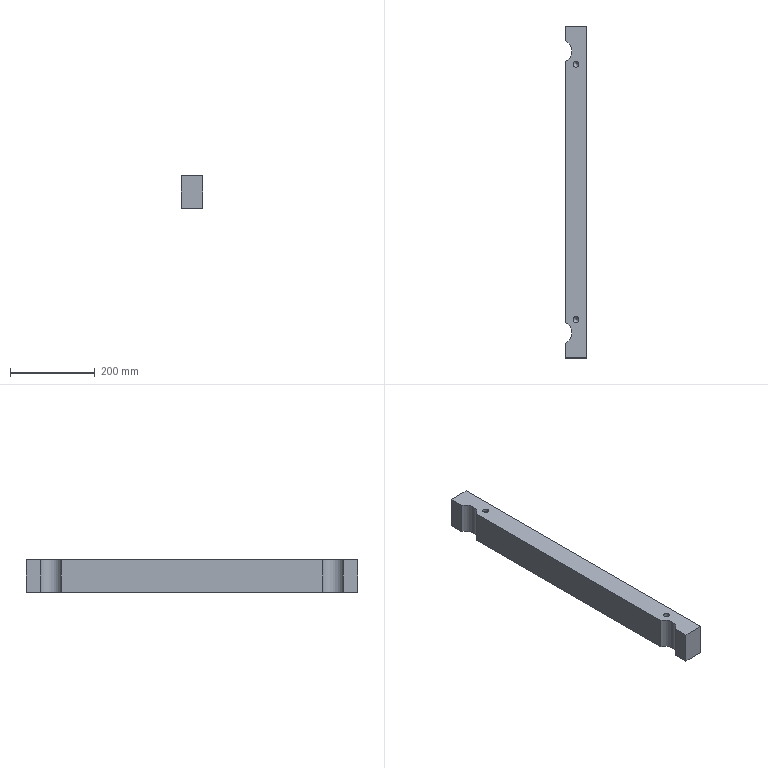Part | NX | features 3 2 | 1 solid | 14 faces | box 50 x 782.437 x 75.5 mm | volume 2869350 mm3 | plane 8 | cylinder 4 | cone 2 | commonest cylinder face diameters 14.1 x2 53 x2
STEP:
#1=CARTESIAN_POINT('',(2467.05,301.218,256.5));
#2=VERTEX_POINT('',#1);
#3=CARTESIAN_POINT('',(2460.,301.218,256.5));
#4=DIRECTION('',(0.,0.,-1.));
#5=DIRECTION('',(1.,0.,0.));
#6=AXIS2_PLACEMENT_3D('',#3,#4,#5);
#7=CIRCLE('',#6,7.05);
#8=EDGE_CURVE('',#2,#2,#7,.T.);
#9=ORIENTED_EDGE('',*,*,#8,.T.);
#10=EDGE_LOOP('',(#9));
#11=FACE_BOUND('',#10,.T.);
#12=CARTESIAN_POINT('',(2435.,-307.891,256.5));
#13=VERTEX_POINT('',#12);
#14=CARTESIAN_POINT('',(2435.,-356.109,256.5));
#15=VERTEX_POINT('',#14);
#16=CARTESIAN_POINT('',(2424.,-332.,256.5));
#17=DIRECTION('',(0.,0.,-1.));
#18=DIRECTION('',(1.,0.,0.));
#19=AXIS2_PLACEMENT_3D('',#16,#17,#18);
#20=CIRCLE('',#19,26.5);
#21=EDGE_CURVE('',#13,#15,#20,.T.);
#22=ORIENTED_EDGE('',*,*,#21,.T.);
#23=CARTESIAN_POINT('',(2435.,-391.218,256.5));
#24=VERTEX_POINT('',#23);
#25=CARTESIAN_POINT('',(2435.,193.,256.5));
#26=DIRECTION('',(0.,1.,0.));
#27=VECTOR('',#26,1000.);
#28=LINE('',#25,#27);
#29=EDGE_CURVE('',#24,#15,#28,.T.);
#30=ORIENTED_EDGE('',*,*,#29,.F.);
#31=CARTESIAN_POINT('',(2485.,-391.218,256.5));
#32=VERTEX_POINT('',#31);
#33=CARTESIAN_POINT('',(4475.,-391.218,256.5));
#34=DIRECTION('',(1.,0.,0.));
#35=VECTOR('',#34,1000.);
#36=LINE('',#33,#35);
#37=EDGE_CURVE('',#24,#32,#36,.T.);
#38=ORIENTED_EDGE('',*,*,#37,.T.);
#39=CARTESIAN_POINT('',(2485.,391.218,256.5));
#40=VERTEX_POINT('',#39);
#41=CARTESIAN_POINT('',(2485.,193.,256.5));
#42=DIRECTION('',(0.,-1.,0.));
#43=VECTOR('',#42,1000.);
#44=LINE('',#41,#43);
#45=EDGE_CURVE('',#40,#32,#44,.T.);
#46=ORIENTED_EDGE('',*,*,#45,.F.);
#47=CARTESIAN_POINT('',(2435.,391.218,256.5));
#48=VERTEX_POINT('',#47);
#49=CARTESIAN_POINT('',(4475.,391.218,256.5));
#50=DIRECTION('',(1.,0.,0.));
#51=VECTOR('',#50,1000.);
#52=LINE('',#49,#51);
#53=EDGE_CURVE('',#48,#40,#52,.T.);
#54=ORIENTED_EDGE('',*,*,#53,.F.);
#55=CARTESIAN_POINT('',(2435.,356.109,256.5));
#56=VERTEX_POINT('',#55);
#57=CARTESIAN_POINT('',(2435.,193.,256.5));
#58=DIRECTION('',(0.,1.,0.));
#59=VECTOR('',#58,1000.);
#60=LINE('',#57,#59);
#61=EDGE_CURVE('',#56,#48,#60,.T.);
#62=ORIENTED_EDGE('',*,*,#61,.F.);
#63=CARTESIAN_POINT('',(2435.,307.891,256.5));
#64=VERTEX_POINT('',#63);
#65=CARTESIAN_POINT('',(2424.,332.,256.5));
#66=DIRECTION('',(0.,0.,1.));
#67=DIRECTION('',(1.,0.,0.));
#68=AXIS2_PLACEMENT_3D('',#65,#66,#67);
#69=CIRCLE('',#68,26.5);
#70=EDGE_CURVE('',#64,#56,#69,.T.);
#71=ORIENTED_EDGE('',*,*,#70,.F.);
#72=CARTESIAN_POINT('',(2435.,193.,256.5));
#73=DIRECTION('',(0.,1.,0.));
#74=VECTOR('',#73,1000.);
#75=LINE('',#72,#74);
#76=EDGE_CURVE('',#13,#64,#75,.T.);
#77=ORIENTED_EDGE('',*,*,#76,.F.);
#78=EDGE_LOOP('',(#22,#30,#38,#46,#54,#62,#71,#77));
#79=FACE_BOUND('',#78,.T.);
#80=CARTESIAN_POINT('',(2467.05,-301.218,256.5));
#81=VERTEX_POINT('',#80);
#82=CARTESIAN_POINT('',(2460.,-301.218,256.5));
#83=DIRECTION('',(0.,0.,-1.));
#84=DIRECTION('',(1.,0.,0.));
#85=AXIS2_PLACEMENT_3D('',#82,#83,#84);
#86=CIRCLE('',#85,7.05);
#87=EDGE_CURVE('',#81,#81,#86,.T.);
#88=ORIENTED_EDGE('',*,*,#87,.T.);
#89=EDGE_LOOP('',(#88));
#90=FACE_BOUND('',#89,.T.);
#91=CARTESIAN_POINT('',(4475.,0.,256.5));
#92=DIRECTION('',(0.,0.,1.));
#93=DIRECTION('',(-1.,0.,0.));
#94=AXIS2_PLACEMENT_3D('',#91,#92,#93);
#95=PLANE('',#94);
#96=ADVANCED_FACE('',(#11,#79,#90),#95,.T.);
#97=CARTESIAN_POINT('',(2435.,-356.109,181.));
#98=VERTEX_POINT('',#97);
#99=CARTESIAN_POINT('',(2435.,-356.109,-181.));
#100=DIRECTION('',(0.,0.,-1.));
#101=VECTOR('',#100,1000.);
#102=LINE('',#99,#101);
#103=EDGE_CURVE('',#15,#98,#102,.T.);
#104=ORIENTED_EDGE('',*,*,#103,.T.);
#105=CARTESIAN_POINT('',(2435.,-391.218,181.));
#106=VERTEX_POINT('',#105);
#107=CARTESIAN_POINT('',(2435.,193.,181.));
#108=DIRECTION('',(0.,-1.,0.));
#109=VECTOR('',#108,1000.);
#110=LINE('',#107,#109);
#111=EDGE_CURVE('',#98,#106,#110,.T.);
#112=ORIENTED_EDGE('',*,*,#111,.T.);
#113=CARTESIAN_POINT('',(2435.,-391.218,-1.5));
#114=DIRECTION('',(0.,0.,1.));
#115=VECTOR('',#114,1000.);
#116=LINE('',#113,#115);
#117=EDGE_CURVE('',#106,#24,#116,.T.);
#118=ORIENTED_EDGE('',*,*,#117,.T.);
#119=ORIENTED_EDGE('',*,*,#29,.T.);
#120=EDGE_LOOP('',(#104,#112,#118,#119));
#121=FACE_BOUND('',#120,.T.);
#122=CARTESIAN_POINT('',(2435.,193.,-1.5));
#123=DIRECTION('',(-1.,0.,0.));
#124=DIRECTION('',(0.,0.,-1.));
#125=AXIS2_PLACEMENT_3D('',#122,#123,#124);
#126=PLANE('',#125);
#127=ADVANCED_FACE('',(#121),#126,.T.);
#128=CARTESIAN_POINT('',(2435.,-307.891,181.));
#129=VERTEX_POINT('',#128);
#130=CARTESIAN_POINT('',(2435.,-307.891,181.));
#131=DIRECTION('',(0.,0.,1.));
#132=VECTOR('',#131,1000.);
#133=LINE('',#130,#132);
#134=EDGE_CURVE('',#129,#13,#133,.T.);
#135=ORIENTED_EDGE('',*,*,#134,.T.);
#136=ORIENTED_EDGE('',*,*,#76,.T.);
#137=CARTESIAN_POINT('',(2435.,307.891,181.));
#138=VERTEX_POINT('',#137);
#139=CARTESIAN_POINT('',(2435.,307.891,-181.));
#140=DIRECTION('',(0.,0.,-1.));
#141=VECTOR('',#140,1000.);
#142=LINE('',#139,#141);
#143=EDGE_CURVE('',#64,#138,#142,.T.);
#144=ORIENTED_EDGE('',*,*,#143,.T.);
#145=CARTESIAN_POINT('',(2435.,193.,181.));
#146=DIRECTION('',(0.,-1.,0.));
#147=VECTOR('',#146,1000.);
#148=LINE('',#145,#147);
#149=EDGE_CURVE('',#138,#129,#148,.T.);
#150=ORIENTED_EDGE('',*,*,#149,.T.);
#151=EDGE_LOOP('',(#135,#136,#144,#150));
#152=FACE_BOUND('',#151,.T.);
#153=CARTESIAN_POINT('',(2435.,193.,-1.5));
#154=DIRECTION('',(-1.,0.,0.));
#155=DIRECTION('',(0.,0.,-1.));
#156=AXIS2_PLACEMENT_3D('',#153,#154,#155);
#157=PLANE('',#156);
#158=ADVANCED_FACE('',(#152),#157,.T.);
#159=CARTESIAN_POINT('',(2435.,356.109,181.));
#160=VERTEX_POINT('',#159);
#161=CARTESIAN_POINT('',(2435.,356.109,181.));
#162=DIRECTION('',(0.,0.,1.));
#163=VECTOR('',#162,1000.);
#164=LINE('',#161,#163);
#165=EDGE_CURVE('',#160,#56,#164,.T.);
#166=ORIENTED_EDGE('',*,*,#165,.T.);
#167=ORIENTED_EDGE('',*,*,#61,.T.);
#168=CARTESIAN_POINT('',(2435.,391.218,181.));
#169=VERTEX_POINT('',#168);
#170=CARTESIAN_POINT('',(2435.,391.218,-1.5));
#171=DIRECTION('',(0.,0.,1.));
#172=VECTOR('',#171,1000.);
#173=LINE('',#170,#172);
#174=EDGE_CURVE('',#169,#48,#173,.T.);
#175=ORIENTED_EDGE('',*,*,#174,.F.);
#176=CARTESIAN_POINT('',(2435.,193.,181.));
#177=DIRECTION('',(0.,-1.,0.));
#178=VECTOR('',#177,1000.);
#179=LINE('',#176,#178);
#180=EDGE_CURVE('',#169,#160,#179,.T.);
#181=ORIENTED_EDGE('',*,*,#180,.T.);
#182=EDGE_LOOP('',(#166,#167,#175,#181));
#183=FACE_BOUND('',#182,.T.);
#184=CARTESIAN_POINT('',(2435.,193.,-1.5));
#185=DIRECTION('',(-1.,0.,0.));
#186=DIRECTION('',(0.,0.,-1.));
#187=AXIS2_PLACEMENT_3D('',#184,#185,#186);
#188=PLANE('',#187);
#189=ADVANCED_FACE('',(#183),#188,.T.);
#190=CARTESIAN_POINT('',(2485.,-391.218,181.));
#191=VERTEX_POINT('',#190);
#192=CARTESIAN_POINT('',(2485.,391.218,181.));
#193=VERTEX_POINT('',#192);
#194=CARTESIAN_POINT('',(2485.,193.,181.));
#195=DIRECTION('',(0.,1.,0.));
#196=VECTOR('',#195,1000.);
#197=LINE('',#194,#196);
#198=EDGE_CURVE('',#191,#193,#197,.T.);
#199=ORIENTED_EDGE('',*,*,#198,.T.);
#200=CARTESIAN_POINT('',(2485.,391.218,-1.5));
#201=DIRECTION('',(0.,0.,-1.));
#202=VECTOR('',#201,1000.);
#203=LINE('',#200,#202);
#204=EDGE_CURVE('',#40,#193,#203,.T.);
#205=ORIENTED_EDGE('',*,*,#204,.F.);
#206=ORIENTED_EDGE('',*,*,#45,.T.);
#207=CARTESIAN_POINT('',(2485.,-391.218,-1.5));
#208=DIRECTION('',(0.,0.,-1.));
#209=VECTOR('',#208,1000.);
#210=LINE('',#207,#209);
#211=EDGE_CURVE('',#32,#191,#210,.T.);
#212=ORIENTED_EDGE('',*,*,#211,.T.);
#213=EDGE_LOOP('',(#199,#205,#206,#212));
#214=FACE_BOUND('',#213,.T.);
#215=CARTESIAN_POINT('',(2485.,193.,-1.5));
#216=DIRECTION('',(1.,0.,0.));
#217=DIRECTION('',(0.,0.,1.));
#218=AXIS2_PLACEMENT_3D('',#215,#216,#217);
#219=PLANE('',#218);
#220=ADVANCED_FACE('',(#214),#219,.T.);
#221=CARTESIAN_POINT('',(2424.,-332.,181.));
#222=DIRECTION('',(0.,0.,-1.));
#223=DIRECTION('',(-1.,0.,0.));
#224=AXIS2_PLACEMENT_3D('',#221,#222,#223);
#225=CIRCLE('',#224,26.5);
#226=EDGE_CURVE('',#129,#98,#225,.T.);
#227=ORIENTED_EDGE('',*,*,#226,.F.);
#228=ORIENTED_EDGE('',*,*,#149,.F.);
#229=CARTESIAN_POINT('',(2424.,332.,181.));
#230=DIRECTION('',(0.,0.,1.));
#231=DIRECTION('',(-1.,0.,0.));
#232=AXIS2_PLACEMENT_3D('',#229,#230,#231);
#233=CIRCLE('',#232,26.5);
#234=EDGE_CURVE('',#138,#160,#233,.T.);
#235=ORIENTED_EDGE('',*,*,#234,.T.);
#236=ORIENTED_EDGE('',*,*,#180,.F.);
#237=CARTESIAN_POINT('',(3705.,391.218,181.));
#238=DIRECTION('',(-1.,0.,0.));
#239=VECTOR('',#238,1000.);
#240=LINE('',#237,#239);
#241=EDGE_CURVE('',#193,#169,#240,.T.);
#242=ORIENTED_EDGE('',*,*,#241,.F.);
#243=ORIENTED_EDGE('',*,*,#198,.F.);
#244=CARTESIAN_POINT('',(3705.,-391.218,181.));
#245=DIRECTION('',(-1.,0.,0.));
#246=VECTOR('',#245,1000.);
#247=LINE('',#244,#246);
#248=EDGE_CURVE('',#191,#106,#247,.T.);
#249=ORIENTED_EDGE('',*,*,#248,.T.);
#250=ORIENTED_EDGE('',*,*,#111,.F.);
#251=EDGE_LOOP('',(#227,#228,#235,#236,#242,#243,#249,#250));
#252=FACE_BOUND('',#251,.T.);
#253=CARTESIAN_POINT('',(3705.,193.,181.));
#254=DIRECTION('',(0.,0.,-1.));
#255=DIRECTION('',(-1.,0.,0.));
#256=AXIS2_PLACEMENT_3D('',#253,#254,#255);
#257=PLANE('',#256);
#258=ADVANCED_FACE('',(#252),#257,.T.);
#259=ORIENTED_EDGE('',*,*,#37,.F.);
#260=ORIENTED_EDGE('',*,*,#117,.F.);
#261=ORIENTED_EDGE('',*,*,#248,.F.);
#262=ORIENTED_EDGE('',*,*,#211,.F.);
#263=EDGE_LOOP('',(#259,#260,#261,#262));
#264=FACE_BOUND('',#263,.T.);
#265=CARTESIAN_POINT('',(2283.371,-391.218,0.));
#266=DIRECTION('',(0.,-1.,0.));
#267=DIRECTION('',(0.,0.,1.));
#268=AXIS2_PLACEMENT_3D('',#265,#266,#267);
#269=PLANE('',#268);
#270=ADVANCED_FACE('',(#264),#269,.T.);
#271=ORIENTED_EDGE('',*,*,#53,.T.);
#272=ORIENTED_EDGE('',*,*,#204,.T.);
#273=ORIENTED_EDGE('',*,*,#241,.T.);
#274=ORIENTED_EDGE('',*,*,#174,.T.);
#275=EDGE_LOOP('',(#271,#272,#273,#274));
#276=FACE_BOUND('',#275,.T.);
#277=CARTESIAN_POINT('',(2283.371,391.218,0.));
#278=DIRECTION('',(0.,1.,0.));
#279=DIRECTION('',(0.,0.,1.));
#280=AXIS2_PLACEMENT_3D('',#277,#278,#279);
#281=PLANE('',#280);
#282=ADVANCED_FACE('',(#276),#281,.T.);
#283=ORIENTED_EDGE('',*,*,#70,.T.);
#284=ORIENTED_EDGE('',*,*,#165,.F.);
#285=ORIENTED_EDGE('',*,*,#234,.F.);
#286=ORIENTED_EDGE('',*,*,#143,.F.);
#287=EDGE_LOOP('',(#283,#284,#285,#286));
#288=FACE_BOUND('',#287,.T.);
#289=CARTESIAN_POINT('',(2424.,332.,-181.));
#290=DIRECTION('',(0.,0.,1.));
#291=DIRECTION('',(-1.,0.,0.));
#292=AXIS2_PLACEMENT_3D('',#289,#290,#291);
#293=CYLINDRICAL_SURFACE('',#292,26.5);
#294=ADVANCED_FACE('',(#288),#293,.F.);
#295=ORIENTED_EDGE('',*,*,#21,.F.);
#296=ORIENTED_EDGE('',*,*,#134,.F.);
#297=ORIENTED_EDGE('',*,*,#226,.T.);
#298=ORIENTED_EDGE('',*,*,#103,.F.);
#299=EDGE_LOOP('',(#295,#296,#297,#298));
#300=FACE_BOUND('',#299,.T.);
#301=CARTESIAN_POINT('',(2424.,-332.,-181.));
#302=DIRECTION('',(0.,0.,1.));
#303=DIRECTION('',(-1.,0.,0.));
#304=AXIS2_PLACEMENT_3D('',#301,#302,#303);
#305=CYLINDRICAL_SURFACE('',#304,26.5);
#306=ADVANCED_FACE('',(#300),#305,.F.);
#307=CARTESIAN_POINT('',(2452.95,301.218,248.55));
#308=VERTEX_POINT('',#307);
#309=CARTESIAN_POINT('',(2460.,301.218,248.55));
#310=DIRECTION('',(0.,0.,-1.));
#311=DIRECTION('',(-1.,0.,0.));
#312=AXIS2_PLACEMENT_3D('',#309,#310,#311);
#313=CIRCLE('',#312,7.05);
#314=EDGE_CURVE('',#308,#308,#313,.T.);
#315=ORIENTED_EDGE('',*,*,#314,.T.);
#316=EDGE_LOOP('',(#315));
#317=FACE_BOUND('',#316,.T.);
#318=ORIENTED_EDGE('',*,*,#8,.F.);
#319=EDGE_LOOP('',(#318));
#320=FACE_BOUND('',#319,.T.);
#321=CARTESIAN_POINT('',(2460.,301.218,256.5));
#322=DIRECTION('',(0.,0.,-1.));
#323=DIRECTION('',(-1.,0.,0.));
#324=AXIS2_PLACEMENT_3D('',#321,#322,#323);
#325=CYLINDRICAL_SURFACE('',#324,7.05);
#326=ADVANCED_FACE('',(#317,#320),#325,.F.);
#327=CARTESIAN_POINT('',(2460.,301.218,241.5));
#328=VERTEX_POINT('',#327);
#329=VERTEX_LOOP('',#328);
#330=FACE_BOUND('',#329,.T.);
#331=ORIENTED_EDGE('',*,*,#314,.F.);
#332=EDGE_LOOP('',(#331));
#333=FACE_BOUND('',#332,.T.);
#334=CARTESIAN_POINT('',(2460.,301.218,248.55));
#335=DIRECTION('',(0.,0.,1.));
#336=DIRECTION('',(-1.,0.,0.));
#337=AXIS2_PLACEMENT_3D('',#334,#335,#336);
#338=CONICAL_SURFACE('',#337,7.05,0.7854);
#339=ADVANCED_FACE('',(#330,#333),#338,.F.);
#340=CARTESIAN_POINT('',(2452.95,-301.218,248.55));
#341=VERTEX_POINT('',#340);
#342=CARTESIAN_POINT('',(2460.,-301.218,248.55));
#343=DIRECTION('',(0.,0.,-1.));
#344=DIRECTION('',(-1.,0.,0.));
#345=AXIS2_PLACEMENT_3D('',#342,#343,#344);
#346=CIRCLE('',#345,7.05);
#347=EDGE_CURVE('',#341,#341,#346,.T.);
#348=ORIENTED_EDGE('',*,*,#347,.T.);
#349=EDGE_LOOP('',(#348));
#350=FACE_BOUND('',#349,.T.);
#351=ORIENTED_EDGE('',*,*,#87,.F.);
#352=EDGE_LOOP('',(#351));
#353=FACE_BOUND('',#352,.T.);
#354=CARTESIAN_POINT('',(2460.,-301.218,256.5));
#355=DIRECTION('',(0.,0.,-1.));
#356=DIRECTION('',(-1.,0.,0.));
#357=AXIS2_PLACEMENT_3D('',#354,#355,#356);
#358=CYLINDRICAL_SURFACE('',#357,7.05);
#359=ADVANCED_FACE('',(#350,#353),#358,.F.);
#360=CARTESIAN_POINT('',(2460.,-301.218,241.5));
#361=VERTEX_POINT('',#360);
#362=VERTEX_LOOP('',#361);
#363=FACE_BOUND('',#362,.T.);
#364=ORIENTED_EDGE('',*,*,#347,.F.);
#365=EDGE_LOOP('',(#364));
#366=FACE_BOUND('',#365,.T.);
#367=CARTESIAN_POINT('',(2460.,-301.218,248.55));
#368=DIRECTION('',(0.,0.,1.));
#369=DIRECTION('',(-1.,0.,0.));
#370=AXIS2_PLACEMENT_3D('',#367,#368,#369);
#371=CONICAL_SURFACE('',#370,7.05,0.7854);
#372=ADVANCED_FACE('',(#363,#366),#371,.F.);
#373=CLOSED_SHELL('',(#96,#127,#158,#189,#220,#258,#270,#282,#294,#306,#326,#339,#359,#372));
#374=MANIFOLD_SOLID_BREP('',#373);
#375=(LENGTH_UNIT()NAMED_UNIT(*)SI_UNIT(.MILLI.,.METRE.));
#376=UNCERTAINTY_MEASURE_WITH_UNIT(LENGTH_MEASURE(0.00001),#375,'','');
#377=(NAMED_UNIT(*)PLANE_ANGLE_UNIT()SI_UNIT($,.RADIAN.));
#378=(NAMED_UNIT(*)SI_UNIT($,.STERADIAN.)SOLID_ANGLE_UNIT());
#379=(GEOMETRIC_REPRESENTATION_CONTEXT(3)GLOBAL_UNCERTAINTY_ASSIGNED_CONTEXT((#376))GLOBAL_UNIT_ASSIGNED_CONTEXT((#375,#377,#378))REPRESENTATION_CONTEXT('',''));
#380=ADVANCED_BREP_SHAPE_REPRESENTATION('',(#374),#379);